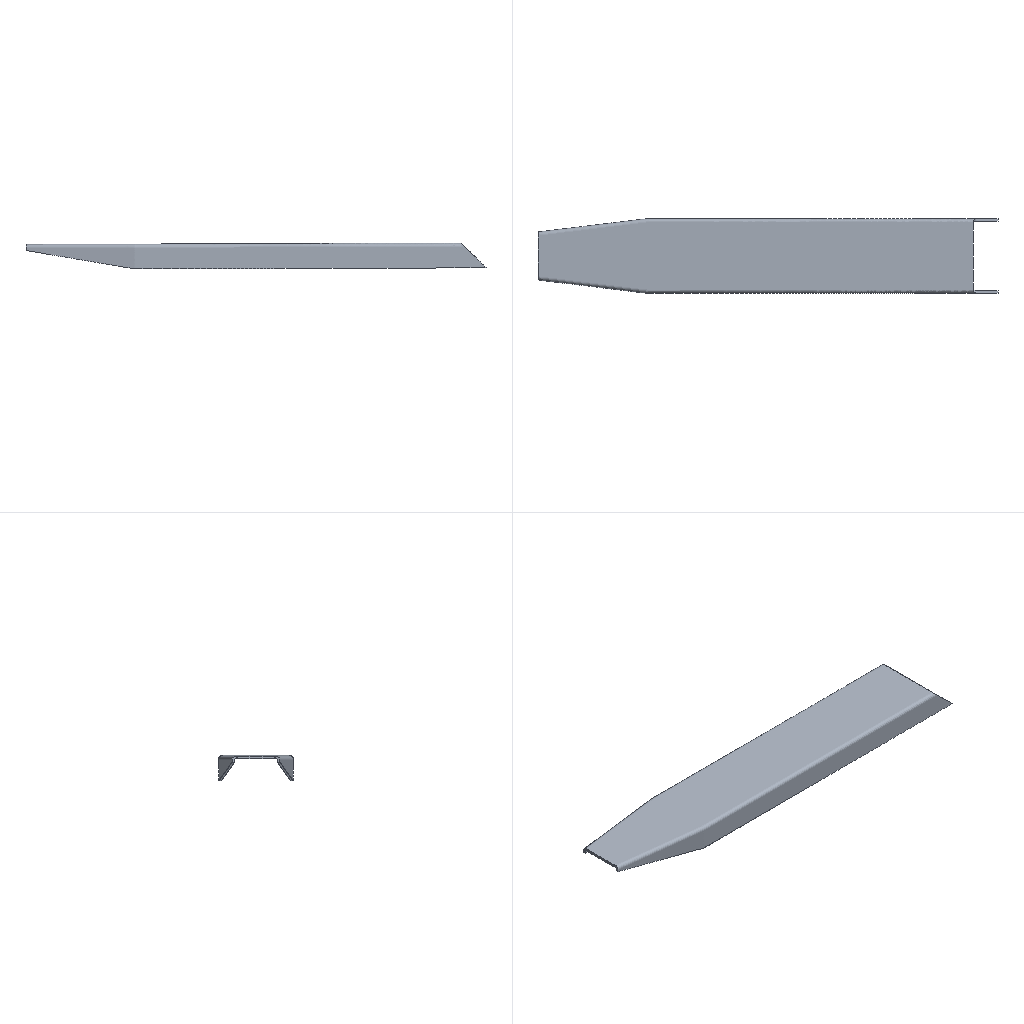Simulation study | nx simcenter
Set-up summary:
category,name,step,type,value,unit,region
solver,nx_nastran (Simcenter)
units,not stated in the deck,,not stated
analysis,deck,,static,static
analysis,solution,,SOL,101
load_step,SUBCASE 1,1,SUBCASE,SPC=1 LOAD=2
load_step,requested,,,1
mesh,nodes,,,269238
mesh,elements,,,141983
element_type,CTETRA,,solid,141983
load,nodal force total,,FX,0.0,model units
load,nodal force total,,FY,0.0,model units
load,nodal force total,,FZ,-2000001.575,model units
load,load commands in deck,,count,129250
bc,support commands in deck,,count,1304
analysis,NX solution 0,,Structural,SESTATIC 101 - Single Constraint
check,setup vs results,,match,every grid point's frame and coordinates and every element id; grid points of CTETRA elements
Nastran input file, long lists of numbers shortened:
$*$$$$$$$$$$$$$$$$$$$$$$$$$$$$$$$$$$$$$$$$$$$$$$$$$$$$$$$$$$$$$$$$$
$*
$*                    Simcenter v12.0.0.27 Translator
$*                    for NX Nastran version 12.0
$ (40 more lines like these left out)
ID,NASTRAN,货叉_sim1-solution_1
SOL 101
CEND
$*
$*$$$$$$$$$$$$$$$$$$$$$$$$$$$$$$$$$$$
$*
$* CASE CONTROL
$*
$*$$$$$$$$$$$$$$$$$$$$$$$$$$$$$$$$$$$
$*
ECHO = NONE
SPC = 1
OUTPUT
DISPLACEMENT(PLOT,REAL) = ALL
SPCFORCES(PLOT,REAL) = ALL
STRESS(PLOT,REAL,VONMISES,CENTER) = ALL
$*  Step: Subcase - Static Loads 1
SUBCASE 1
  LABEL = Subcase - Static Loads 1
  LOAD = 2
$*
$*$$$$$$$$$$$$$$$$$$$$$$$$$$$$$$$$$$$
$*
$* BULK DATA
$*
$*$$$$$$$$$$$$$$$$$$$$$$$$$$$$$$$$$$$
$*
BEGIN BULK
$*
$* PARAM CARDS
$*
PARAM      K6ROT100.0000
PARAM     OIBULK     YES
PARAM    OMACHPR     YES
PARAM       POST      -2
PARAM    POSTEXT     YES
PARAM    UNITSYS   MN-MM
$*
$* GRID CARDS
$*
GRID*                  1               0-3.691982177E+02-2.914311468E+02+
*       -1.118703209E+02               0
GRID*                  2               0-3.686640027E+02-2.913229347E+02+
*       -1.093689184E+02               0
$ (538472 more lines like these left out)
$*
$* ELEMENT CARDS
$*
$*  Mesh Collector: Solid(1)
$*  Mesh: 3d_mesh(1)
CTETRA         1       1  245068       1  245075       2    4584    4585+
+         256165    4586    4587    4588
CTETRA         2       1  245069  245074       3       2  256160    4589+
+           4590    4591    4592    4593
$ (283962 more lines like these left out)
$*
$* PROPERTY CARDS
$*
$*  Property: PSOLID1
PSOLID         1       1       0                           SMECH
$*
$* MATERIAL CARDS
$*
$*  Material: Steel::货叉_fem1::[1]
MAT1           12.0694+8        0.2880007.8290-61.1280-5
MATT1          1       1               2               3
TABLEM1        1                       1                                +
+        20.00002.0694+8 21.11002.0694+8    ENDT
TABLEM1        2                       1                                +
+        20.00000.288000 21.11000.288000 23.89000.288000 37.78000.288000+
+        51.67000.289000 65.56000.289000 79.44000.290000 93.33000.290000+
+       107.22000.291000121.11000.291000135.00000.291000148.89000.292000+
+       162.78000.292000176.67000.293000190.56000.293000204.44000.293000+
+       218.33000.294000232.22000.294000246.11000.294000260.00000.295000+
+       273.89000.295000287.78000.296000301.67000.296000315.56000.296000+
+       329.44000.297000343.33000.297000357.22000.298000371.11000.298000+
+       385.00000.298000398.89000.299000412.78000.299000426.67000.300000+
+       440.56000.300000454.44000.301000468.33000.301000482.22000.302000+
+       496.11000.302000510.00000.303000523.89000.304000537.78000.304000+
+       551.67000.305000565.56000.306000579.44000.307000593.33000.308000+
+       607.22000.309000621.11000.310000635.00000.311000648.89000.312000+
+       662.78000.313000676.67000.314000690.56000.316000704.44000.317000+
+           ENDT
TABLEM1        3                       1                                +
+        20.00001.1280-5 93.33001.1790-5107.22001.1880-5121.11001.1970-5+
+       135.00001.2060-5148.89001.2132-5162.78001.2222-5176.67001.2312-5+
+       190.56001.2402-5204.44001.2492-5218.33001.2582-5232.22001.2672-5+
+       246.11001.2762-5260.00001.2852-5273.89001.2942-5287.78001.3032-5+
+       301.67001.3122-5315.56001.3212-5329.44001.3302-5343.33001.3392-5+
+       357.22001.3464-5371.11001.3554-5385.00001.3644-5398.89001.3734-5+
+       412.78001.3806-5426.67001.3896-5440.56001.3986-5454.44001.4058-5+
+       468.33001.4148-5482.22001.4238-5496.11001.4310-5510.00001.4400-5+
+       523.89001.4472-5537.78001.4544-5551.67001.4616-5565.56001.4688-5+
+       579.44001.4742-5593.33001.4796-5607.22001.4832-5621.11001.4886-5+
+       635.00001.4904-5648.89001.4922-5662.78001.4922-5676.67001.4922-5+
+       690.56001.4904-5704.44001.4886-5718.33001.4850-5732.22001.4796-5+
+       746.11001.4724-5760.00001.4634-5773.89001.4472-5787.78001.4256-5+
+       801.67001.4004-5815.56001.3680-5    ENDT
$*
$* LOAD AND CONSTRAINT CARDS
$*
$*  Constraint: Fixed(1)
SPC            1  210624  123456  0.0000
SPC            1  210625  123456  0.0000
SPC            1  210626  123456  0.0000
SPC            1  210627  123456  0.0000
$ (1300 more lines like these left out)
$*  Load: Force(1)
FORCE          2       1       0 15.4739  0.0000  0.0000-1.00000
FORCE          2       2       0 15.4739  0.0000  0.0000-1.00000
FORCE          2       3       0 15.4739  0.0000  0.0000-1.00000
FORCE          2       4       0 15.4739  0.0000  0.0000-1.00000
$ (129246 more lines like these left out)
ENDDATA 17f422f3
Results summary:
result,analysis,,,static
result,last_loadstep,,,1
result,primary field,,,displacements
result,reaction total,,FX,-3.549,model units
result,reaction total,,FY,0.2151,model units
result,reaction total,,FZ,2000002.125,model units
result,NX solution 0,,loadcases,1,mm